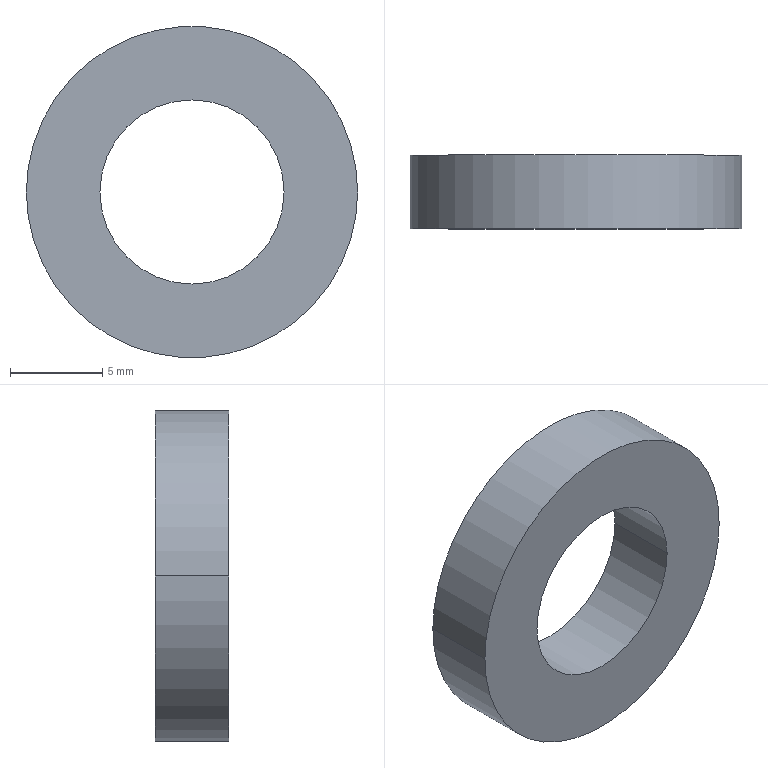Part | SolidWorks | features Revolution 1 | 1 solid | 6 faces | box 18 x 4 x 18 mm | volume 703.717 mm3 | cylinder 4 | plane 2 | commonest cylinder face diameters 10 x2 18 x2
STEP:
#1=CARTESIAN_POINT('',(9.,0.,0.));
#2=VERTEX_POINT('',#1);
#3=CARTESIAN_POINT('',(-9.,0.,0.));
#4=VERTEX_POINT('',#3);
#5=CARTESIAN_POINT('',(0.,0.,0.));
#6=DIRECTION('',(0.,-1.,0.));
#7=DIRECTION('',(1.,0.,0.));
#8=AXIS2_PLACEMENT_3D('',#5,#6,#7);
#9=CIRCLE('',#8,9.);
#10=EDGE_CURVE('',#2,#4,#9,.T.);
#11=ORIENTED_EDGE('',*,*,#10,.T.);
#12=CARTESIAN_POINT('',(-9.,-4.,0.));
#13=VERTEX_POINT('',#12);
#14=CARTESIAN_POINT('',(-9.,-473.381,0.));
#15=DIRECTION('',(0.,-1.,0.));
#16=VECTOR('',#15,1000.);
#17=LINE('',#14,#16);
#18=EDGE_CURVE('',#4,#13,#17,.T.);
#19=ORIENTED_EDGE('',*,*,#18,.T.);
#20=CARTESIAN_POINT('',(9.,-4.,0.));
#21=VERTEX_POINT('',#20);
#22=CARTESIAN_POINT('',(0.,-4.,0.));
#23=DIRECTION('',(0.,-1.,0.));
#24=DIRECTION('',(1.,0.,0.));
#25=AXIS2_PLACEMENT_3D('',#22,#23,#24);
#26=CIRCLE('',#25,9.);
#27=EDGE_CURVE('',#21,#13,#26,.T.);
#28=ORIENTED_EDGE('',*,*,#27,.F.);
#29=CARTESIAN_POINT('',(9.,-473.381,0.));
#30=DIRECTION('',(0.,-1.,0.));
#31=VECTOR('',#30,1000.);
#32=LINE('',#29,#31);
#33=EDGE_CURVE('',#2,#21,#32,.T.);
#34=ORIENTED_EDGE('',*,*,#33,.F.);
#35=EDGE_LOOP('',(#11,#19,#28,#34));
#36=FACE_OUTER_BOUND('',#35,.T.);
#37=CARTESIAN_POINT('',(0.,-473.381,0.));
#38=DIRECTION('',(0.,-1.,0.));
#39=DIRECTION('',(1.,0.,0.));
#40=AXIS2_PLACEMENT_3D('',#37,#38,#39);
#41=CYLINDRICAL_SURFACE('',#40,9.);
#42=ADVANCED_FACE('',(#36),#41,.T.);
#43=CARTESIAN_POINT('',(-5.,0.,0.));
#44=VERTEX_POINT('',#43);
#45=CARTESIAN_POINT('',(5.,0.,0.));
#46=VERTEX_POINT('',#45);
#47=CARTESIAN_POINT('',(0.,0.,0.));
#48=DIRECTION('',(0.,-1.,0.));
#49=DIRECTION('',(1.,0.,0.));
#50=AXIS2_PLACEMENT_3D('',#47,#48,#49);
#51=CIRCLE('',#50,5.);
#52=EDGE_CURVE('',#44,#46,#51,.T.);
#53=ORIENTED_EDGE('',*,*,#52,.F.);
#54=CARTESIAN_POINT('',(-5.,-4.,0.));
#55=VERTEX_POINT('',#54);
#56=CARTESIAN_POINT('',(-5.,-473.381,0.));
#57=DIRECTION('',(0.,-1.,0.));
#58=VECTOR('',#57,1000.);
#59=LINE('',#56,#58);
#60=EDGE_CURVE('',#44,#55,#59,.T.);
#61=ORIENTED_EDGE('',*,*,#60,.T.);
#62=CARTESIAN_POINT('',(5.,-4.,0.));
#63=VERTEX_POINT('',#62);
#64=CARTESIAN_POINT('',(0.,-4.,0.));
#65=DIRECTION('',(0.,-1.,0.));
#66=DIRECTION('',(1.,0.,0.));
#67=AXIS2_PLACEMENT_3D('',#64,#65,#66);
#68=CIRCLE('',#67,5.);
#69=EDGE_CURVE('',#55,#63,#68,.T.);
#70=ORIENTED_EDGE('',*,*,#69,.T.);
#71=CARTESIAN_POINT('',(5.,-473.381,0.));
#72=DIRECTION('',(0.,-1.,0.));
#73=VECTOR('',#72,1000.);
#74=LINE('',#71,#73);
#75=EDGE_CURVE('',#46,#63,#74,.T.);
#76=ORIENTED_EDGE('',*,*,#75,.F.);
#77=EDGE_LOOP('',(#53,#61,#70,#76));
#78=FACE_OUTER_BOUND('',#77,.T.);
#79=CARTESIAN_POINT('',(0.,-473.381,0.));
#80=DIRECTION('',(0.,-1.,0.));
#81=DIRECTION('',(1.,0.,0.));
#82=AXIS2_PLACEMENT_3D('',#79,#80,#81);
#83=CYLINDRICAL_SURFACE('',#82,5.);
#84=ADVANCED_FACE('',(#78),#83,.F.);
#85=ORIENTED_EDGE('',*,*,#60,.F.);
#86=CARTESIAN_POINT('',(0.,0.,0.));
#87=DIRECTION('',(0.,-1.,0.));
#88=DIRECTION('',(1.,0.,0.));
#89=AXIS2_PLACEMENT_3D('',#86,#87,#88);
#90=CIRCLE('',#89,5.);
#91=EDGE_CURVE('',#46,#44,#90,.T.);
#92=ORIENTED_EDGE('',*,*,#91,.F.);
#93=ORIENTED_EDGE('',*,*,#75,.T.);
#94=CARTESIAN_POINT('',(0.,-4.,0.));
#95=DIRECTION('',(0.,-1.,0.));
#96=DIRECTION('',(1.,0.,0.));
#97=AXIS2_PLACEMENT_3D('',#94,#95,#96);
#98=CIRCLE('',#97,5.);
#99=EDGE_CURVE('',#63,#55,#98,.T.);
#100=ORIENTED_EDGE('',*,*,#99,.T.);
#101=EDGE_LOOP('',(#85,#92,#93,#100));
#102=FACE_OUTER_BOUND('',#101,.T.);
#103=CARTESIAN_POINT('',(0.,-473.381,0.));
#104=DIRECTION('',(0.,-1.,0.));
#105=DIRECTION('',(1.,0.,0.));
#106=AXIS2_PLACEMENT_3D('',#103,#104,#105);
#107=CYLINDRICAL_SURFACE('',#106,5.);
#108=ADVANCED_FACE('',(#102),#107,.F.);
#109=ORIENTED_EDGE('',*,*,#27,.T.);
#110=CARTESIAN_POINT('',(0.,-4.,0.));
#111=DIRECTION('',(0.,-1.,0.));
#112=DIRECTION('',(1.,0.,0.));
#113=AXIS2_PLACEMENT_3D('',#110,#111,#112);
#114=CIRCLE('',#113,9.);
#115=EDGE_CURVE('',#13,#21,#114,.T.);
#116=ORIENTED_EDGE('',*,*,#115,.T.);
#117=EDGE_LOOP('',(#109,#116));
#118=FACE_OUTER_BOUND('',#117,.T.);
#119=ORIENTED_EDGE('',*,*,#99,.F.);
#120=ORIENTED_EDGE('',*,*,#69,.F.);
#121=EDGE_LOOP('',(#119,#120));
#122=FACE_BOUND('',#121,.T.);
#123=CARTESIAN_POINT('',(5.,-4.,0.));
#124=DIRECTION('',(0.,-1.,0.));
#125=DIRECTION('',(1.,0.,0.));
#126=AXIS2_PLACEMENT_3D('',#123,#124,#125);
#127=PLANE('',#126);
#128=ADVANCED_FACE('',(#118,#122),#127,.T.);
#129=ORIENTED_EDGE('',*,*,#18,.F.);
#130=CARTESIAN_POINT('',(0.,0.,0.));
#131=DIRECTION('',(0.,-1.,0.));
#132=DIRECTION('',(1.,0.,0.));
#133=AXIS2_PLACEMENT_3D('',#130,#131,#132);
#134=CIRCLE('',#133,9.);
#135=EDGE_CURVE('',#4,#2,#134,.T.);
#136=ORIENTED_EDGE('',*,*,#135,.T.);
#137=ORIENTED_EDGE('',*,*,#33,.T.);
#138=ORIENTED_EDGE('',*,*,#115,.F.);
#139=EDGE_LOOP('',(#129,#136,#137,#138));
#140=FACE_OUTER_BOUND('',#139,.T.);
#141=CARTESIAN_POINT('',(0.,-473.381,0.));
#142=DIRECTION('',(0.,-1.,0.));
#143=DIRECTION('',(1.,0.,0.));
#144=AXIS2_PLACEMENT_3D('',#141,#142,#143);
#145=CYLINDRICAL_SURFACE('',#144,9.);
#146=ADVANCED_FACE('',(#140),#145,.T.);
#147=ORIENTED_EDGE('',*,*,#91,.T.);
#148=ORIENTED_EDGE('',*,*,#52,.T.);
#149=EDGE_LOOP('',(#147,#148));
#150=FACE_BOUND('',#149,.T.);
#151=ORIENTED_EDGE('',*,*,#10,.F.);
#152=ORIENTED_EDGE('',*,*,#135,.F.);
#153=EDGE_LOOP('',(#151,#152));
#154=FACE_OUTER_BOUND('',#153,.T.);
#155=CARTESIAN_POINT('',(5.,0.,0.));
#156=DIRECTION('',(0.,1.,0.));
#157=DIRECTION('',(-1.,0.,0.));
#158=AXIS2_PLACEMENT_3D('',#155,#156,#157);
#159=PLANE('',#158);
#160=ADVANCED_FACE('',(#150,#154),#159,.T.);
#161=CLOSED_SHELL('',(#42,#84,#108,#128,#146,#160));
#162=MANIFOLD_SOLID_BREP('',#161);
#163=CARTESIAN_POINT('',(0.,0.,0.));
#164=DIRECTION('',(0.,0.,1.));
#165=DIRECTION('',(1.,0.,0.));
#166=AXIS2_PLACEMENT_3D('',#163,#164,#165);
#167=(LENGTH_UNIT()NAMED_UNIT(*)SI_UNIT(.MILLI.,.METRE.));
#168=UNCERTAINTY_MEASURE_WITH_UNIT(LENGTH_MEASURE(0.00001),#167,'','');
#169=(NAMED_UNIT(*)PLANE_ANGLE_UNIT()SI_UNIT($,.RADIAN.));
#170=(NAMED_UNIT(*)SI_UNIT($,.STERADIAN.)SOLID_ANGLE_UNIT());
#171=(GEOMETRIC_REPRESENTATION_CONTEXT(3)GLOBAL_UNCERTAINTY_ASSIGNED_CONTEXT((#168))GLOBAL_UNIT_ASSIGNED_CONTEXT((#167,#169,#170))REPRESENTATION_CONTEXT('',''));
#172=ADVANCED_BREP_SHAPE_REPRESENTATION('',(#162,#166),#171);